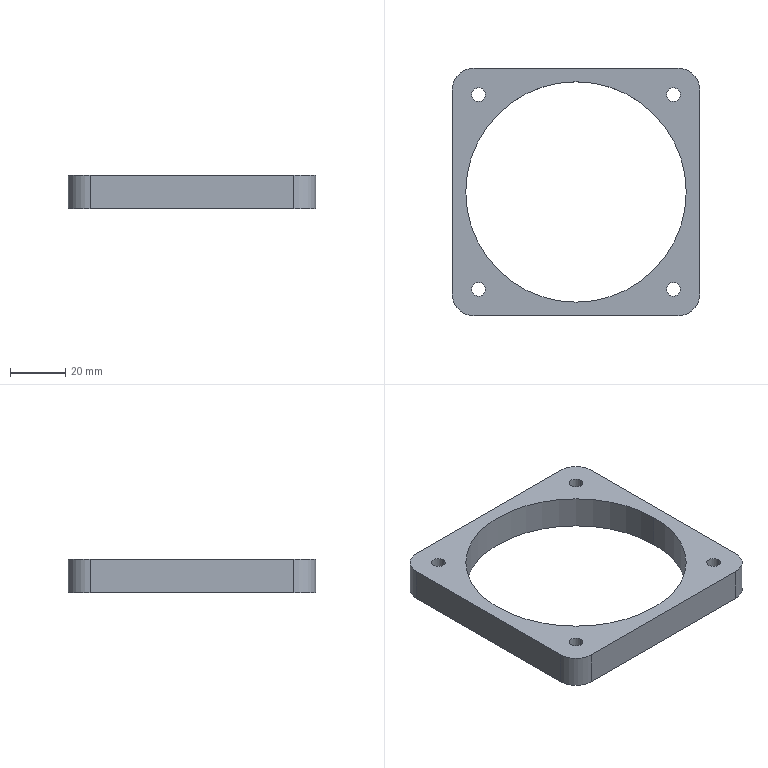Part | SolidWorks | features FlatPattern 1, HoleWzd 1, SMBaseFlange 1, SheetMetal 1 | 1 solid | 20 faces | box 90 x 90 x 12 mm | volume 35280 mm3 | cylinder 14 | plane 6 | commonest cylinder face diameters 5 x8 16 x4 80 x2
STEP:
#1=CARTESIAN_POINT('',(20027.498,-16996.803,-12.));
#2=VERTEX_POINT('',#1);
#3=CARTESIAN_POINT('',(20032.498,-16996.803,-12.));
#4=VERTEX_POINT('',#3);
#5=CARTESIAN_POINT('',(20029.998,-16996.803,-12.));
#6=DIRECTION('',(0.,0.,1.));
#7=DIRECTION('',(1.,0.,0.));
#8=AXIS2_PLACEMENT_3D('',#5,#6,#7);
#9=CIRCLE('',#8,2.5);
#10=EDGE_CURVE('',#2,#4,#9,.T.);
#11=ORIENTED_EDGE('',*,*,#10,.F.);
#12=CARTESIAN_POINT('',(20027.498,-16996.803,0.));
#13=VERTEX_POINT('',#12);
#14=CARTESIAN_POINT('',(20027.498,-16996.803,0.));
#15=DIRECTION('',(0.,0.,1.));
#16=VECTOR('',#15,1000.);
#17=LINE('',#14,#16);
#18=EDGE_CURVE('',#2,#13,#17,.T.);
#19=ORIENTED_EDGE('',*,*,#18,.T.);
#20=CARTESIAN_POINT('',(20032.498,-16996.803,0.));
#21=VERTEX_POINT('',#20);
#22=CARTESIAN_POINT('',(20029.998,-16996.803,0.));
#23=DIRECTION('',(0.,0.,1.));
#24=DIRECTION('',(1.,0.,0.));
#25=AXIS2_PLACEMENT_3D('',#22,#23,#24);
#26=CIRCLE('',#25,2.5);
#27=EDGE_CURVE('',#13,#21,#26,.T.);
#28=ORIENTED_EDGE('',*,*,#27,.T.);
#29=CARTESIAN_POINT('',(20032.498,-16996.803,0.));
#30=DIRECTION('',(0.,0.,1.));
#31=VECTOR('',#30,1000.);
#32=LINE('',#29,#31);
#33=EDGE_CURVE('',#4,#21,#32,.T.);
#34=ORIENTED_EDGE('',*,*,#33,.F.);
#35=EDGE_LOOP('',(#11,#19,#28,#34));
#36=FACE_OUTER_BOUND('',#35,.T.);
#37=CARTESIAN_POINT('',(20029.998,-16996.803,0.));
#38=DIRECTION('',(0.,0.,1.));
#39=DIRECTION('',(1.,0.,0.));
#40=AXIS2_PLACEMENT_3D('',#37,#38,#39);
#41=CYLINDRICAL_SURFACE('',#40,2.5);
#42=ADVANCED_FACE('',(#36),#41,.F.);
#43=CARTESIAN_POINT('',(20098.208,-16996.803,-12.));
#44=VERTEX_POINT('',#43);
#45=CARTESIAN_POINT('',(20103.208,-16996.803,-12.));
#46=VERTEX_POINT('',#45);
#47=CARTESIAN_POINT('',(20100.708,-16996.803,-12.));
#48=DIRECTION('',(0.,0.,1.));
#49=DIRECTION('',(1.,0.,0.));
#50=AXIS2_PLACEMENT_3D('',#47,#48,#49);
#51=CIRCLE('',#50,2.5);
#52=EDGE_CURVE('',#44,#46,#51,.T.);
#53=ORIENTED_EDGE('',*,*,#52,.F.);
#54=CARTESIAN_POINT('',(20098.208,-16996.803,0.));
#55=VERTEX_POINT('',#54);
#56=CARTESIAN_POINT('',(20098.208,-16996.803,0.));
#57=DIRECTION('',(0.,0.,1.));
#58=VECTOR('',#57,1000.);
#59=LINE('',#56,#58);
#60=EDGE_CURVE('',#44,#55,#59,.T.);
#61=ORIENTED_EDGE('',*,*,#60,.T.);
#62=CARTESIAN_POINT('',(20103.208,-16996.803,0.));
#63=VERTEX_POINT('',#62);
#64=CARTESIAN_POINT('',(20100.708,-16996.803,0.));
#65=DIRECTION('',(0.,0.,1.));
#66=DIRECTION('',(1.,0.,0.));
#67=AXIS2_PLACEMENT_3D('',#64,#65,#66);
#68=CIRCLE('',#67,2.5);
#69=EDGE_CURVE('',#55,#63,#68,.T.);
#70=ORIENTED_EDGE('',*,*,#69,.T.);
#71=CARTESIAN_POINT('',(20103.208,-16996.803,0.));
#72=DIRECTION('',(0.,0.,1.));
#73=VECTOR('',#72,1000.);
#74=LINE('',#71,#73);
#75=EDGE_CURVE('',#46,#63,#74,.T.);
#76=ORIENTED_EDGE('',*,*,#75,.F.);
#77=EDGE_LOOP('',(#53,#61,#70,#76));
#78=FACE_OUTER_BOUND('',#77,.T.);
#79=CARTESIAN_POINT('',(20100.708,-16996.803,0.));
#80=DIRECTION('',(0.,0.,1.));
#81=DIRECTION('',(1.,0.,0.));
#82=AXIS2_PLACEMENT_3D('',#79,#80,#81);
#83=CYLINDRICAL_SURFACE('',#82,2.5);
#84=ADVANCED_FACE('',(#78),#83,.F.);
#85=CARTESIAN_POINT('',(20098.208,-17067.514,-12.));
#86=VERTEX_POINT('',#85);
#87=CARTESIAN_POINT('',(20103.208,-17067.514,-12.));
#88=VERTEX_POINT('',#87);
#89=CARTESIAN_POINT('',(20100.708,-17067.514,-12.));
#90=DIRECTION('',(0.,0.,1.));
#91=DIRECTION('',(1.,0.,0.));
#92=AXIS2_PLACEMENT_3D('',#89,#90,#91);
#93=CIRCLE('',#92,2.5);
#94=EDGE_CURVE('',#86,#88,#93,.T.);
#95=ORIENTED_EDGE('',*,*,#94,.F.);
#96=CARTESIAN_POINT('',(20098.208,-17067.514,0.));
#97=VERTEX_POINT('',#96);
#98=CARTESIAN_POINT('',(20098.208,-17067.514,0.));
#99=DIRECTION('',(0.,0.,1.));
#100=VECTOR('',#99,1000.);
#101=LINE('',#98,#100);
#102=EDGE_CURVE('',#86,#97,#101,.T.);
#103=ORIENTED_EDGE('',*,*,#102,.T.);
#104=CARTESIAN_POINT('',(20103.208,-17067.514,0.));
#105=VERTEX_POINT('',#104);
#106=CARTESIAN_POINT('',(20100.708,-17067.514,0.));
#107=DIRECTION('',(0.,0.,1.));
#108=DIRECTION('',(1.,0.,0.));
#109=AXIS2_PLACEMENT_3D('',#106,#107,#108);
#110=CIRCLE('',#109,2.5);
#111=EDGE_CURVE('',#97,#105,#110,.T.);
#112=ORIENTED_EDGE('',*,*,#111,.T.);
#113=CARTESIAN_POINT('',(20103.208,-17067.514,0.));
#114=DIRECTION('',(0.,0.,1.));
#115=VECTOR('',#114,1000.);
#116=LINE('',#113,#115);
#117=EDGE_CURVE('',#88,#105,#116,.T.);
#118=ORIENTED_EDGE('',*,*,#117,.F.);
#119=EDGE_LOOP('',(#95,#103,#112,#118));
#120=FACE_OUTER_BOUND('',#119,.T.);
#121=CARTESIAN_POINT('',(20100.708,-17067.514,0.));
#122=DIRECTION('',(0.,0.,1.));
#123=DIRECTION('',(1.,0.,0.));
#124=AXIS2_PLACEMENT_3D('',#121,#122,#123);
#125=CYLINDRICAL_SURFACE('',#124,2.5);
#126=ADVANCED_FACE('',(#120),#125,.F.);
#127=CARTESIAN_POINT('',(20027.498,-17067.514,-12.));
#128=VERTEX_POINT('',#127);
#129=CARTESIAN_POINT('',(20032.498,-17067.514,-12.));
#130=VERTEX_POINT('',#129);
#131=CARTESIAN_POINT('',(20029.998,-17067.514,-12.));
#132=DIRECTION('',(0.,0.,1.));
#133=DIRECTION('',(1.,0.,0.));
#134=AXIS2_PLACEMENT_3D('',#131,#132,#133);
#135=CIRCLE('',#134,2.5);
#136=EDGE_CURVE('',#128,#130,#135,.T.);
#137=ORIENTED_EDGE('',*,*,#136,.F.);
#138=CARTESIAN_POINT('',(20027.498,-17067.514,0.));
#139=VERTEX_POINT('',#138);
#140=CARTESIAN_POINT('',(20027.498,-17067.514,0.));
#141=DIRECTION('',(0.,0.,1.));
#142=VECTOR('',#141,1000.);
#143=LINE('',#140,#142);
#144=EDGE_CURVE('',#128,#139,#143,.T.);
#145=ORIENTED_EDGE('',*,*,#144,.T.);
#146=CARTESIAN_POINT('',(20032.498,-17067.514,0.));
#147=VERTEX_POINT('',#146);
#148=CARTESIAN_POINT('',(20029.998,-17067.514,0.));
#149=DIRECTION('',(0.,0.,1.));
#150=DIRECTION('',(1.,0.,0.));
#151=AXIS2_PLACEMENT_3D('',#148,#149,#150);
#152=CIRCLE('',#151,2.5);
#153=EDGE_CURVE('',#139,#147,#152,.T.);
#154=ORIENTED_EDGE('',*,*,#153,.T.);
#155=CARTESIAN_POINT('',(20032.498,-17067.514,0.));
#156=DIRECTION('',(0.,0.,1.));
#157=VECTOR('',#156,1000.);
#158=LINE('',#155,#157);
#159=EDGE_CURVE('',#130,#147,#158,.T.);
#160=ORIENTED_EDGE('',*,*,#159,.F.);
#161=EDGE_LOOP('',(#137,#145,#154,#160));
#162=FACE_OUTER_BOUND('',#161,.T.);
#163=CARTESIAN_POINT('',(20029.998,-17067.514,0.));
#164=DIRECTION('',(0.,0.,1.));
#165=DIRECTION('',(1.,0.,0.));
#166=AXIS2_PLACEMENT_3D('',#163,#164,#165);
#167=CYLINDRICAL_SURFACE('',#166,2.5);
#168=ADVANCED_FACE('',(#162),#167,.F.);
#169=CARTESIAN_POINT('',(20025.353,-17032.159,-12.));
#170=VERTEX_POINT('',#169);
#171=CARTESIAN_POINT('',(20105.353,-17032.159,-12.));
#172=VERTEX_POINT('',#171);
#173=CARTESIAN_POINT('',(20065.353,-17032.159,-12.));
#174=DIRECTION('',(0.,0.,1.));
#175=DIRECTION('',(1.,0.,0.));
#176=AXIS2_PLACEMENT_3D('',#173,#174,#175);
#177=CIRCLE('',#176,40.);
#178=EDGE_CURVE('',#170,#172,#177,.T.);
#179=ORIENTED_EDGE('',*,*,#178,.F.);
#180=CARTESIAN_POINT('',(20025.353,-17032.159,0.));
#181=VERTEX_POINT('',#180);
#182=CARTESIAN_POINT('',(20025.353,-17032.159,-12.));
#183=DIRECTION('',(0.,0.,1.));
#184=VECTOR('',#183,1000.);
#185=LINE('',#182,#184);
#186=EDGE_CURVE('',#170,#181,#185,.T.);
#187=ORIENTED_EDGE('',*,*,#186,.T.);
#188=CARTESIAN_POINT('',(20105.353,-17032.159,0.));
#189=VERTEX_POINT('',#188);
#190=CARTESIAN_POINT('',(20065.353,-17032.159,0.));
#191=DIRECTION('',(0.,0.,1.));
#192=DIRECTION('',(1.,0.,0.));
#193=AXIS2_PLACEMENT_3D('',#190,#191,#192);
#194=CIRCLE('',#193,40.);
#195=EDGE_CURVE('',#181,#189,#194,.T.);
#196=ORIENTED_EDGE('',*,*,#195,.T.);
#197=CARTESIAN_POINT('',(20105.353,-17032.159,-12.));
#198=DIRECTION('',(0.,0.,1.));
#199=VECTOR('',#198,1000.);
#200=LINE('',#197,#199);
#201=EDGE_CURVE('',#172,#189,#200,.T.);
#202=ORIENTED_EDGE('',*,*,#201,.F.);
#203=EDGE_LOOP('',(#179,#187,#196,#202));
#204=FACE_OUTER_BOUND('',#203,.T.);
#205=CARTESIAN_POINT('',(20065.353,-17032.159,-12.));
#206=DIRECTION('',(0.,0.,1.));
#207=DIRECTION('',(1.,0.,0.));
#208=AXIS2_PLACEMENT_3D('',#205,#206,#207);
#209=CYLINDRICAL_SURFACE('',#208,40.);
#210=ADVANCED_FACE('',(#204),#209,.F.);
#211=CARTESIAN_POINT('',(20020.353,-17069.159,0.));
#212=VERTEX_POINT('',#211);
#213=CARTESIAN_POINT('',(20028.353,-17077.159,0.));
#214=VERTEX_POINT('',#213);
#215=CARTESIAN_POINT('',(20028.353,-17069.159,0.));
#216=DIRECTION('',(0.,0.,1.));
#217=DIRECTION('',(1.,0.,0.));
#218=AXIS2_PLACEMENT_3D('',#215,#216,#217);
#219=CIRCLE('',#218,8.);
#220=EDGE_CURVE('',#212,#214,#219,.T.);
#221=ORIENTED_EDGE('',*,*,#220,.F.);
#222=CARTESIAN_POINT('',(20020.353,-17069.159,-12.));
#223=VERTEX_POINT('',#222);
#224=CARTESIAN_POINT('',(20020.353,-17069.159,-12.));
#225=DIRECTION('',(0.,0.,1.));
#226=VECTOR('',#225,1000.);
#227=LINE('',#224,#226);
#228=EDGE_CURVE('',#223,#212,#227,.T.);
#229=ORIENTED_EDGE('',*,*,#228,.F.);
#230=CARTESIAN_POINT('',(20028.353,-17077.159,-12.));
#231=VERTEX_POINT('',#230);
#232=CARTESIAN_POINT('',(20028.353,-17069.159,-12.));
#233=DIRECTION('',(0.,0.,1.));
#234=DIRECTION('',(1.,0.,0.));
#235=AXIS2_PLACEMENT_3D('',#232,#233,#234);
#236=CIRCLE('',#235,8.);
#237=EDGE_CURVE('',#223,#231,#236,.T.);
#238=ORIENTED_EDGE('',*,*,#237,.T.);
#239=CARTESIAN_POINT('',(20028.353,-17077.159,-12.));
#240=DIRECTION('',(0.,0.,1.));
#241=VECTOR('',#240,1000.);
#242=LINE('',#239,#241);
#243=EDGE_CURVE('',#231,#214,#242,.T.);
#244=ORIENTED_EDGE('',*,*,#243,.T.);
#245=EDGE_LOOP('',(#221,#229,#238,#244));
#246=FACE_OUTER_BOUND('',#245,.T.);
#247=CARTESIAN_POINT('',(20028.353,-17069.159,-12.));
#248=DIRECTION('',(0.,0.,1.));
#249=DIRECTION('',(1.,0.,0.));
#250=AXIS2_PLACEMENT_3D('',#247,#248,#249);
#251=CYLINDRICAL_SURFACE('',#250,8.);
#252=ADVANCED_FACE('',(#246),#251,.T.);
#253=CARTESIAN_POINT('',(20020.353,-16995.159,0.));
#254=VERTEX_POINT('',#253);
#255=CARTESIAN_POINT('',(20020.353,-17069.159,0.));
#256=DIRECTION('',(0.,-1.,0.));
#257=VECTOR('',#256,1000.);
#258=LINE('',#255,#257);
#259=EDGE_CURVE('',#254,#212,#258,.T.);
#260=ORIENTED_EDGE('',*,*,#259,.F.);
#261=CARTESIAN_POINT('',(20020.353,-16995.159,-12.));
#262=VERTEX_POINT('',#261);
#263=CARTESIAN_POINT('',(20020.353,-16995.159,-12.));
#264=DIRECTION('',(0.,0.,1.));
#265=VECTOR('',#264,1000.);
#266=LINE('',#263,#265);
#267=EDGE_CURVE('',#262,#254,#266,.T.);
#268=ORIENTED_EDGE('',*,*,#267,.F.);
#269=CARTESIAN_POINT('',(20020.353,-17069.159,-12.));
#270=DIRECTION('',(0.,-1.,0.));
#271=VECTOR('',#270,1000.);
#272=LINE('',#269,#271);
#273=EDGE_CURVE('',#262,#223,#272,.T.);
#274=ORIENTED_EDGE('',*,*,#273,.T.);
#275=ORIENTED_EDGE('',*,*,#228,.T.);
#276=EDGE_LOOP('',(#260,#268,#274,#275));
#277=FACE_OUTER_BOUND('',#276,.T.);
#278=CARTESIAN_POINT('',(20020.353,-17069.159,-12.));
#279=DIRECTION('',(-1.,0.,0.));
#280=DIRECTION('',(0.,0.,1.));
#281=AXIS2_PLACEMENT_3D('',#278,#279,#280);
#282=PLANE('',#281);
#283=ADVANCED_FACE('',(#277),#282,.T.);
#284=CARTESIAN_POINT('',(20028.353,-16987.159,0.));
#285=VERTEX_POINT('',#284);
#286=CARTESIAN_POINT('',(20028.353,-16995.159,0.));
#287=DIRECTION('',(0.,0.,1.));
#288=DIRECTION('',(1.,0.,0.));
#289=AXIS2_PLACEMENT_3D('',#286,#287,#288);
#290=CIRCLE('',#289,8.);
#291=EDGE_CURVE('',#285,#254,#290,.T.);
#292=ORIENTED_EDGE('',*,*,#291,.F.);
#293=CARTESIAN_POINT('',(20028.353,-16987.159,-12.));
#294=VERTEX_POINT('',#293);
#295=CARTESIAN_POINT('',(20028.353,-16987.159,-12.));
#296=DIRECTION('',(0.,0.,1.));
#297=VECTOR('',#296,1000.);
#298=LINE('',#295,#297);
#299=EDGE_CURVE('',#294,#285,#298,.T.);
#300=ORIENTED_EDGE('',*,*,#299,.F.);
#301=CARTESIAN_POINT('',(20028.353,-16995.159,-12.));
#302=DIRECTION('',(0.,0.,1.));
#303=DIRECTION('',(1.,0.,0.));
#304=AXIS2_PLACEMENT_3D('',#301,#302,#303);
#305=CIRCLE('',#304,8.);
#306=EDGE_CURVE('',#294,#262,#305,.T.);
#307=ORIENTED_EDGE('',*,*,#306,.T.);
#308=ORIENTED_EDGE('',*,*,#267,.T.);
#309=EDGE_LOOP('',(#292,#300,#307,#308));
#310=FACE_OUTER_BOUND('',#309,.T.);
#311=CARTESIAN_POINT('',(20028.353,-16995.159,-12.));
#312=DIRECTION('',(0.,0.,1.));
#313=DIRECTION('',(1.,0.,0.));
#314=AXIS2_PLACEMENT_3D('',#311,#312,#313);
#315=CYLINDRICAL_SURFACE('',#314,8.);
#316=ADVANCED_FACE('',(#310),#315,.T.);
#317=CARTESIAN_POINT('',(20102.353,-16987.159,0.));
#318=VERTEX_POINT('',#317);
#319=CARTESIAN_POINT('',(20028.353,-16987.159,0.));
#320=DIRECTION('',(-1.,0.,0.));
#321=VECTOR('',#320,1000.);
#322=LINE('',#319,#321);
#323=EDGE_CURVE('',#318,#285,#322,.T.);
#324=ORIENTED_EDGE('',*,*,#323,.F.);
#325=CARTESIAN_POINT('',(20102.353,-16987.159,-12.));
#326=VERTEX_POINT('',#325);
#327=CARTESIAN_POINT('',(20102.353,-16987.159,-12.));
#328=DIRECTION('',(0.,0.,1.));
#329=VECTOR('',#328,1000.);
#330=LINE('',#327,#329);
#331=EDGE_CURVE('',#326,#318,#330,.T.);
#332=ORIENTED_EDGE('',*,*,#331,.F.);
#333=CARTESIAN_POINT('',(20028.353,-16987.159,-12.));
#334=DIRECTION('',(-1.,0.,0.));
#335=VECTOR('',#334,1000.);
#336=LINE('',#333,#335);
#337=EDGE_CURVE('',#326,#294,#336,.T.);
#338=ORIENTED_EDGE('',*,*,#337,.T.);
#339=ORIENTED_EDGE('',*,*,#299,.T.);
#340=EDGE_LOOP('',(#324,#332,#338,#339));
#341=FACE_OUTER_BOUND('',#340,.T.);
#342=CARTESIAN_POINT('',(20028.353,-16987.159,-12.));
#343=DIRECTION('',(0.,1.,0.));
#344=DIRECTION('',(0.,0.,1.));
#345=AXIS2_PLACEMENT_3D('',#342,#343,#344);
#346=PLANE('',#345);
#347=ADVANCED_FACE('',(#341),#346,.T.);
#348=CARTESIAN_POINT('',(20110.353,-16995.159,0.));
#349=VERTEX_POINT('',#348);
#350=CARTESIAN_POINT('',(20102.353,-16995.159,0.));
#351=DIRECTION('',(0.,0.,1.));
#352=DIRECTION('',(1.,0.,0.));
#353=AXIS2_PLACEMENT_3D('',#350,#351,#352);
#354=CIRCLE('',#353,8.);
#355=EDGE_CURVE('',#349,#318,#354,.T.);
#356=ORIENTED_EDGE('',*,*,#355,.F.);
#357=CARTESIAN_POINT('',(20110.353,-16995.159,-12.));
#358=VERTEX_POINT('',#357);
#359=CARTESIAN_POINT('',(20110.353,-16995.159,-12.));
#360=DIRECTION('',(0.,0.,1.));
#361=VECTOR('',#360,1000.);
#362=LINE('',#359,#361);
#363=EDGE_CURVE('',#358,#349,#362,.T.);
#364=ORIENTED_EDGE('',*,*,#363,.F.);
#365=CARTESIAN_POINT('',(20102.353,-16995.159,-12.));
#366=DIRECTION('',(0.,0.,1.));
#367=DIRECTION('',(1.,0.,0.));
#368=AXIS2_PLACEMENT_3D('',#365,#366,#367);
#369=CIRCLE('',#368,8.);
#370=EDGE_CURVE('',#358,#326,#369,.T.);
#371=ORIENTED_EDGE('',*,*,#370,.T.);
#372=ORIENTED_EDGE('',*,*,#331,.T.);
#373=EDGE_LOOP('',(#356,#364,#371,#372));
#374=FACE_OUTER_BOUND('',#373,.T.);
#375=CARTESIAN_POINT('',(20102.353,-16995.159,-12.));
#376=DIRECTION('',(0.,0.,1.));
#377=DIRECTION('',(1.,0.,0.));
#378=AXIS2_PLACEMENT_3D('',#375,#376,#377);
#379=CYLINDRICAL_SURFACE('',#378,8.);
#380=ADVANCED_FACE('',(#374),#379,.T.);
#381=CARTESIAN_POINT('',(20110.353,-17069.159,0.));
#382=VERTEX_POINT('',#381);
#383=CARTESIAN_POINT('',(20110.353,-16995.159,0.));
#384=DIRECTION('',(0.,1.,0.));
#385=VECTOR('',#384,1000.);
#386=LINE('',#383,#385);
#387=EDGE_CURVE('',#382,#349,#386,.T.);
#388=ORIENTED_EDGE('',*,*,#387,.F.);
#389=CARTESIAN_POINT('',(20110.353,-17069.159,-12.));
#390=VERTEX_POINT('',#389);
#391=CARTESIAN_POINT('',(20110.353,-17069.159,-12.));
#392=DIRECTION('',(0.,0.,1.));
#393=VECTOR('',#392,1000.);
#394=LINE('',#391,#393);
#395=EDGE_CURVE('',#390,#382,#394,.T.);
#396=ORIENTED_EDGE('',*,*,#395,.F.);
#397=CARTESIAN_POINT('',(20110.353,-16995.159,-12.));
#398=DIRECTION('',(0.,1.,0.));
#399=VECTOR('',#398,1000.);
#400=LINE('',#397,#399);
#401=EDGE_CURVE('',#390,#358,#400,.T.);
#402=ORIENTED_EDGE('',*,*,#401,.T.);
#403=ORIENTED_EDGE('',*,*,#363,.T.);
#404=EDGE_LOOP('',(#388,#396,#402,#403));
#405=FACE_OUTER_BOUND('',#404,.T.);
#406=CARTESIAN_POINT('',(20110.353,-16995.159,-12.));
#407=DIRECTION('',(1.,0.,0.));
#408=DIRECTION('',(0.,0.,-1.));
#409=AXIS2_PLACEMENT_3D('',#406,#407,#408);
#410=PLANE('',#409);
#411=ADVANCED_FACE('',(#405),#410,.T.);
#412=CARTESIAN_POINT('',(20102.353,-17077.159,0.));
#413=VERTEX_POINT('',#412);
#414=CARTESIAN_POINT('',(20102.353,-17069.159,0.));
#415=DIRECTION('',(0.,0.,1.));
#416=DIRECTION('',(1.,0.,0.));
#417=AXIS2_PLACEMENT_3D('',#414,#415,#416);
#418=CIRCLE('',#417,8.);
#419=EDGE_CURVE('',#413,#382,#418,.T.);
#420=ORIENTED_EDGE('',*,*,#419,.F.);
#421=CARTESIAN_POINT('',(20102.353,-17077.159,-12.));
#422=VERTEX_POINT('',#421);
#423=CARTESIAN_POINT('',(20102.353,-17077.159,-12.));
#424=DIRECTION('',(0.,0.,1.));
#425=VECTOR('',#424,1000.);
#426=LINE('',#423,#425);
#427=EDGE_CURVE('',#422,#413,#426,.T.);
#428=ORIENTED_EDGE('',*,*,#427,.F.);
#429=CARTESIAN_POINT('',(20102.353,-17069.159,-12.));
#430=DIRECTION('',(0.,0.,1.));
#431=DIRECTION('',(1.,0.,0.));
#432=AXIS2_PLACEMENT_3D('',#429,#430,#431);
#433=CIRCLE('',#432,8.);
#434=EDGE_CURVE('',#422,#390,#433,.T.);
#435=ORIENTED_EDGE('',*,*,#434,.T.);
#436=ORIENTED_EDGE('',*,*,#395,.T.);
#437=EDGE_LOOP('',(#420,#428,#435,#436));
#438=FACE_OUTER_BOUND('',#437,.T.);
#439=CARTESIAN_POINT('',(20102.353,-17069.159,-12.));
#440=DIRECTION('',(0.,0.,1.));
#441=DIRECTION('',(1.,0.,0.));
#442=AXIS2_PLACEMENT_3D('',#439,#440,#441);
#443=CYLINDRICAL_SURFACE('',#442,8.);
#444=ADVANCED_FACE('',(#438),#443,.T.);
#445=CARTESIAN_POINT('',(20102.353,-17077.159,0.));
#446=DIRECTION('',(1.,0.,0.));
#447=VECTOR('',#446,1000.);
#448=LINE('',#445,#447);
#449=EDGE_CURVE('',#214,#413,#448,.T.);
#450=ORIENTED_EDGE('',*,*,#449,.F.);
#451=ORIENTED_EDGE('',*,*,#243,.F.);
#452=CARTESIAN_POINT('',(20102.353,-17077.159,-12.));
#453=DIRECTION('',(1.,0.,0.));
#454=VECTOR('',#453,1000.);
#455=LINE('',#452,#454);
#456=EDGE_CURVE('',#231,#422,#455,.T.);
#457=ORIENTED_EDGE('',*,*,#456,.T.);
#458=ORIENTED_EDGE('',*,*,#427,.T.);
#459=EDGE_LOOP('',(#450,#451,#457,#458));
#460=FACE_OUTER_BOUND('',#459,.T.);
#461=CARTESIAN_POINT('',(20102.353,-17077.159,-12.));
#462=DIRECTION('',(0.,-1.,0.));
#463=DIRECTION('',(0.,0.,-1.));
#464=AXIS2_PLACEMENT_3D('',#461,#462,#463);
#465=PLANE('',#464);
#466=ADVANCED_FACE('',(#460),#465,.T.);
#467=CARTESIAN_POINT('',(20029.998,-16996.803,-12.));
#468=DIRECTION('',(0.,0.,1.));
#469=DIRECTION('',(1.,0.,0.));
#470=AXIS2_PLACEMENT_3D('',#467,#468,#469);
#471=CIRCLE('',#470,2.5);
#472=EDGE_CURVE('',#4,#2,#471,.T.);
#473=ORIENTED_EDGE('',*,*,#472,.T.);
#474=ORIENTED_EDGE('',*,*,#10,.T.);
#475=EDGE_LOOP('',(#473,#474));
#476=FACE_BOUND('',#475,.T.);
#477=CARTESIAN_POINT('',(20100.708,-16996.803,-12.));
#478=DIRECTION('',(0.,0.,1.));
#479=DIRECTION('',(1.,0.,0.));
#480=AXIS2_PLACEMENT_3D('',#477,#478,#479);
#481=CIRCLE('',#480,2.5);
#482=EDGE_CURVE('',#46,#44,#481,.T.);
#483=ORIENTED_EDGE('',*,*,#482,.T.);
#484=ORIENTED_EDGE('',*,*,#52,.T.);
#485=EDGE_LOOP('',(#483,#484));
#486=FACE_BOUND('',#485,.T.);
#487=CARTESIAN_POINT('',(20100.708,-17067.514,-12.));
#488=DIRECTION('',(0.,0.,1.));
#489=DIRECTION('',(1.,0.,0.));
#490=AXIS2_PLACEMENT_3D('',#487,#488,#489);
#491=CIRCLE('',#490,2.5);
#492=EDGE_CURVE('',#88,#86,#491,.T.);
#493=ORIENTED_EDGE('',*,*,#492,.T.);
#494=ORIENTED_EDGE('',*,*,#94,.T.);
#495=EDGE_LOOP('',(#493,#494));
#496=FACE_BOUND('',#495,.T.);
#497=CARTESIAN_POINT('',(20029.998,-17067.514,-12.));
#498=DIRECTION('',(0.,0.,1.));
#499=DIRECTION('',(1.,0.,0.));
#500=AXIS2_PLACEMENT_3D('',#497,#498,#499);
#501=CIRCLE('',#500,2.5);
#502=EDGE_CURVE('',#130,#128,#501,.T.);
#503=ORIENTED_EDGE('',*,*,#502,.T.);
#504=ORIENTED_EDGE('',*,*,#136,.T.);
#505=EDGE_LOOP('',(#503,#504));
#506=FACE_BOUND('',#505,.T.);
#507=CARTESIAN_POINT('',(20065.353,-17032.159,-12.));
#508=DIRECTION('',(0.,0.,1.));
#509=DIRECTION('',(1.,0.,0.));
#510=AXIS2_PLACEMENT_3D('',#507,#508,#509);
#511=CIRCLE('',#510,40.);
#512=EDGE_CURVE('',#172,#170,#511,.T.);
#513=ORIENTED_EDGE('',*,*,#512,.T.);
#514=ORIENTED_EDGE('',*,*,#178,.T.);
#515=EDGE_LOOP('',(#513,#514));
#516=FACE_BOUND('',#515,.T.);
#517=ORIENTED_EDGE('',*,*,#237,.F.);
#518=ORIENTED_EDGE('',*,*,#273,.F.);
#519=ORIENTED_EDGE('',*,*,#306,.F.);
#520=ORIENTED_EDGE('',*,*,#337,.F.);
#521=ORIENTED_EDGE('',*,*,#370,.F.);
#522=ORIENTED_EDGE('',*,*,#401,.F.);
#523=ORIENTED_EDGE('',*,*,#434,.F.);
#524=ORIENTED_EDGE('',*,*,#456,.F.);
#525=EDGE_LOOP('',(#517,#518,#519,#520,#521,#522,#523,#524));
#526=FACE_OUTER_BOUND('',#525,.T.);
#527=CARTESIAN_POINT('',(20028.353,-17069.159,-12.));
#528=DIRECTION('',(0.,0.,1.));
#529=DIRECTION('',(1.,0.,0.));
#530=AXIS2_PLACEMENT_3D('',#527,#528,#529);
#531=PLANE('',#530);
#532=ADVANCED_FACE('',(#476,#486,#496,#506,#516,#526),#531,.F.);
#533=CARTESIAN_POINT('',(20029.998,-16996.803,0.));
#534=DIRECTION('',(0.,0.,1.));
#535=DIRECTION('',(1.,0.,0.));
#536=AXIS2_PLACEMENT_3D('',#533,#534,#535);
#537=CIRCLE('',#536,2.5);
#538=EDGE_CURVE('',#21,#13,#537,.T.);
#539=ORIENTED_EDGE('',*,*,#538,.F.);
#540=ORIENTED_EDGE('',*,*,#27,.F.);
#541=EDGE_LOOP('',(#539,#540));
#542=FACE_BOUND('',#541,.T.);
#543=CARTESIAN_POINT('',(20100.708,-16996.803,0.));
#544=DIRECTION('',(0.,0.,1.));
#545=DIRECTION('',(1.,0.,0.));
#546=AXIS2_PLACEMENT_3D('',#543,#544,#545);
#547=CIRCLE('',#546,2.5);
#548=EDGE_CURVE('',#63,#55,#547,.T.);
#549=ORIENTED_EDGE('',*,*,#548,.F.);
#550=ORIENTED_EDGE('',*,*,#69,.F.);
#551=EDGE_LOOP('',(#549,#550));
#552=FACE_BOUND('',#551,.T.);
#553=CARTESIAN_POINT('',(20100.708,-17067.514,0.));
#554=DIRECTION('',(0.,0.,1.));
#555=DIRECTION('',(1.,0.,0.));
#556=AXIS2_PLACEMENT_3D('',#553,#554,#555);
#557=CIRCLE('',#556,2.5);
#558=EDGE_CURVE('',#105,#97,#557,.T.);
#559=ORIENTED_EDGE('',*,*,#558,.F.);
#560=ORIENTED_EDGE('',*,*,#111,.F.);
#561=EDGE_LOOP('',(#559,#560));
#562=FACE_BOUND('',#561,.T.);
#563=CARTESIAN_POINT('',(20029.998,-17067.514,0.));
#564=DIRECTION('',(0.,0.,1.));
#565=DIRECTION('',(1.,0.,0.));
#566=AXIS2_PLACEMENT_3D('',#563,#564,#565);
#567=CIRCLE('',#566,2.5);
#568=EDGE_CURVE('',#147,#139,#567,.T.);
#569=ORIENTED_EDGE('',*,*,#568,.F.);
#570=ORIENTED_EDGE('',*,*,#153,.F.);
#571=EDGE_LOOP('',(#569,#570));
#572=FACE_BOUND('',#571,.T.);
#573=CARTESIAN_POINT('',(20065.353,-17032.159,0.));
#574=DIRECTION('',(0.,0.,1.));
#575=DIRECTION('',(1.,0.,0.));
#576=AXIS2_PLACEMENT_3D('',#573,#574,#575);
#577=CIRCLE('',#576,40.);
#578=EDGE_CURVE('',#189,#181,#577,.T.);
#579=ORIENTED_EDGE('',*,*,#578,.F.);
#580=ORIENTED_EDGE('',*,*,#195,.F.);
#581=EDGE_LOOP('',(#579,#580));
#582=FACE_BOUND('',#581,.T.);
#583=ORIENTED_EDGE('',*,*,#220,.T.);
#584=ORIENTED_EDGE('',*,*,#449,.T.);
#585=ORIENTED_EDGE('',*,*,#419,.T.);
#586=ORIENTED_EDGE('',*,*,#387,.T.);
#587=ORIENTED_EDGE('',*,*,#355,.T.);
#588=ORIENTED_EDGE('',*,*,#323,.T.);
#589=ORIENTED_EDGE('',*,*,#291,.T.);
#590=ORIENTED_EDGE('',*,*,#259,.T.);
#591=EDGE_LOOP('',(#583,#584,#585,#586,#587,#588,#589,#590));
#592=FACE_OUTER_BOUND('',#591,.T.);
#593=CARTESIAN_POINT('',(20028.353,-17069.159,0.));
#594=DIRECTION('',(0.,0.,1.));
#595=DIRECTION('',(1.,0.,0.));
#596=AXIS2_PLACEMENT_3D('',#593,#594,#595);
#597=PLANE('',#596);
#598=ADVANCED_FACE('',(#542,#552,#562,#572,#582,#592),#597,.T.);
#599=ORIENTED_EDGE('',*,*,#186,.F.);
#600=ORIENTED_EDGE('',*,*,#512,.F.);
#601=ORIENTED_EDGE('',*,*,#201,.T.);
#602=ORIENTED_EDGE('',*,*,#578,.T.);
#603=EDGE_LOOP('',(#599,#600,#601,#602));
#604=FACE_OUTER_BOUND('',#603,.T.);
#605=CARTESIAN_POINT('',(20065.353,-17032.159,-12.));
#606=DIRECTION('',(0.,0.,1.));
#607=DIRECTION('',(1.,0.,0.));
#608=AXIS2_PLACEMENT_3D('',#605,#606,#607);
#609=CYLINDRICAL_SURFACE('',#608,40.);
#610=ADVANCED_FACE('',(#604),#609,.F.);
#611=ORIENTED_EDGE('',*,*,#144,.F.);
#612=ORIENTED_EDGE('',*,*,#502,.F.);
#613=ORIENTED_EDGE('',*,*,#159,.T.);
#614=ORIENTED_EDGE('',*,*,#568,.T.);
#615=EDGE_LOOP('',(#611,#612,#613,#614));
#616=FACE_OUTER_BOUND('',#615,.T.);
#617=CARTESIAN_POINT('',(20029.998,-17067.514,0.));
#618=DIRECTION('',(0.,0.,1.));
#619=DIRECTION('',(1.,0.,0.));
#620=AXIS2_PLACEMENT_3D('',#617,#618,#619);
#621=CYLINDRICAL_SURFACE('',#620,2.5);
#622=ADVANCED_FACE('',(#616),#621,.F.);
#623=ORIENTED_EDGE('',*,*,#102,.F.);
#624=ORIENTED_EDGE('',*,*,#492,.F.);
#625=ORIENTED_EDGE('',*,*,#117,.T.);
#626=ORIENTED_EDGE('',*,*,#558,.T.);
#627=EDGE_LOOP('',(#623,#624,#625,#626));
#628=FACE_OUTER_BOUND('',#627,.T.);
#629=CARTESIAN_POINT('',(20100.708,-17067.514,0.));
#630=DIRECTION('',(0.,0.,1.));
#631=DIRECTION('',(1.,0.,0.));
#632=AXIS2_PLACEMENT_3D('',#629,#630,#631);
#633=CYLINDRICAL_SURFACE('',#632,2.5);
#634=ADVANCED_FACE('',(#628),#633,.F.);
#635=ORIENTED_EDGE('',*,*,#60,.F.);
#636=ORIENTED_EDGE('',*,*,#482,.F.);
#637=ORIENTED_EDGE('',*,*,#75,.T.);
#638=ORIENTED_EDGE('',*,*,#548,.T.);
#639=EDGE_LOOP('',(#635,#636,#637,#638));
#640=FACE_OUTER_BOUND('',#639,.T.);
#641=CARTESIAN_POINT('',(20100.708,-16996.803,0.));
#642=DIRECTION('',(0.,0.,1.));
#643=DIRECTION('',(1.,0.,0.));
#644=AXIS2_PLACEMENT_3D('',#641,#642,#643);
#645=CYLINDRICAL_SURFACE('',#644,2.5);
#646=ADVANCED_FACE('',(#640),#645,.F.);
#647=ORIENTED_EDGE('',*,*,#18,.F.);
#648=ORIENTED_EDGE('',*,*,#472,.F.);
#649=ORIENTED_EDGE('',*,*,#33,.T.);
#650=ORIENTED_EDGE('',*,*,#538,.T.);
#651=EDGE_LOOP('',(#647,#648,#649,#650));
#652=FACE_OUTER_BOUND('',#651,.T.);
#653=CARTESIAN_POINT('',(20029.998,-16996.803,0.));
#654=DIRECTION('',(0.,0.,1.));
#655=DIRECTION('',(1.,0.,0.));
#656=AXIS2_PLACEMENT_3D('',#653,#654,#655);
#657=CYLINDRICAL_SURFACE('',#656,2.5);
#658=ADVANCED_FACE('',(#652),#657,.F.);
#659=CLOSED_SHELL('',(#42,#84,#126,#168,#210,#252,#283,#316,#347,#380,#411,#444,#466,#532,#598,#610,#622,#634,#646,#658));
#660=MANIFOLD_SOLID_BREP('',#659);
#661=CARTESIAN_POINT('',(0.,0.,0.));
#662=DIRECTION('',(0.,0.,1.));
#663=DIRECTION('',(1.,0.,0.));
#664=AXIS2_PLACEMENT_3D('',#661,#662,#663);
#665=(LENGTH_UNIT()NAMED_UNIT(*)SI_UNIT(.MILLI.,.METRE.));
#666=UNCERTAINTY_MEASURE_WITH_UNIT(LENGTH_MEASURE(0.00001),#665,'','');
#667=(NAMED_UNIT(*)PLANE_ANGLE_UNIT()SI_UNIT($,.RADIAN.));
#668=(NAMED_UNIT(*)SI_UNIT($,.STERADIAN.)SOLID_ANGLE_UNIT());
#669=(GEOMETRIC_REPRESENTATION_CONTEXT(3)GLOBAL_UNCERTAINTY_ASSIGNED_CONTEXT((#666))GLOBAL_UNIT_ASSIGNED_CONTEXT((#665,#667,#668))REPRESENTATION_CONTEXT('',''));
#670=ADVANCED_BREP_SHAPE_REPRESENTATION('',(#660,#664),#669);